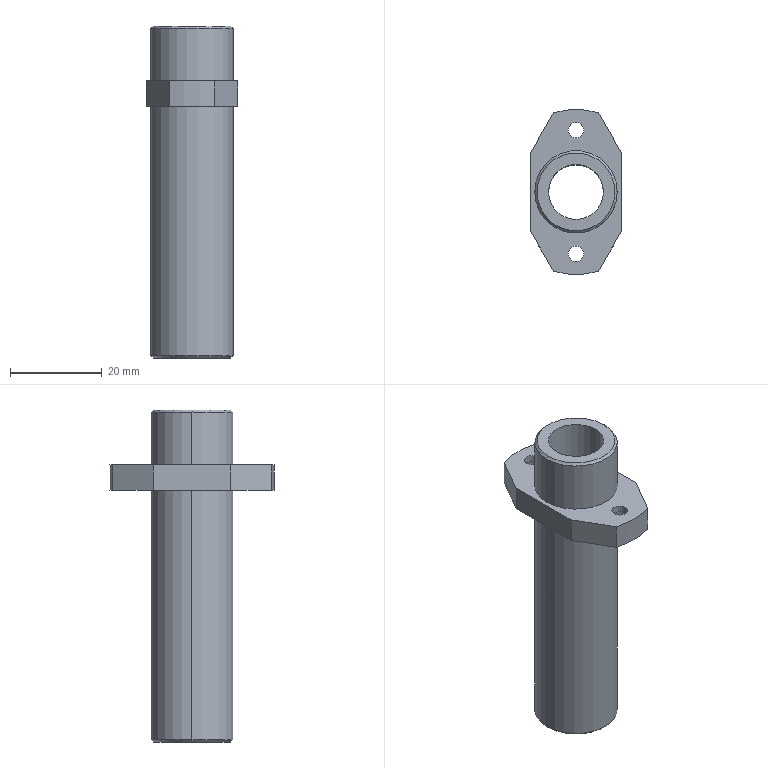Part | STEP file | PN_0016 Default | 1 solid | 38 faces | box 20 x 36 x 72.5 mm | volume 11823 mm3 | cylinder 16 | plane 12 | cone 6 | torus 4 | commonest cylinder face diameters 3.4 x4 6.5 x4 18 x4 12 x2 36 x2
STEP:
#1=CARTESIAN_POINT('',(-7.356,0.,-59.75));
#2=VERTEX_POINT('',#1);
#3=CARTESIAN_POINT('',(7.356,0.,-59.75));
#4=VERTEX_POINT('',#3);
#5=CARTESIAN_POINT('',(0.,0.,-59.75));
#6=DIRECTION('',(0.,0.,-1.));
#7=DIRECTION('',(1.,0.,0.));
#8=AXIS2_PLACEMENT_3D('',#5,#6,#7);
#9=CIRCLE('',#8,7.356);
#10=EDGE_CURVE('',#2,#4,#9,.T.);
#11=ORIENTED_EDGE('',*,*,#10,.F.);
#12=CARTESIAN_POINT('',(-7.789,0.,-60.));
#13=VERTEX_POINT('',#12);
#14=CARTESIAN_POINT('',(-7.789,0.,-59.5));
#15=DIRECTION('',(0.,1.,0.));
#16=DIRECTION('',(-1.,0.,0.));
#17=AXIS2_PLACEMENT_3D('',#14,#15,#16);
#18=CIRCLE('',#17,0.5);
#19=EDGE_CURVE('',#2,#13,#18,.T.);
#20=ORIENTED_EDGE('',*,*,#19,.T.);
#21=CARTESIAN_POINT('',(7.789,0.,-60.));
#22=VERTEX_POINT('',#21);
#23=CARTESIAN_POINT('',(0.,0.,-60.));
#24=DIRECTION('',(0.,0.,1.));
#25=DIRECTION('',(1.,0.,0.));
#26=AXIS2_PLACEMENT_3D('',#23,#24,#25);
#27=CIRCLE('',#26,7.789);
#28=EDGE_CURVE('',#22,#13,#27,.T.);
#29=ORIENTED_EDGE('',*,*,#28,.F.);
#30=CARTESIAN_POINT('',(7.789,0.,-59.5));
#31=DIRECTION('',(0.,-1.,0.));
#32=DIRECTION('',(0.,0.,-1.));
#33=AXIS2_PLACEMENT_3D('',#30,#31,#32);
#34=CIRCLE('',#33,0.5);
#35=EDGE_CURVE('',#4,#22,#34,.T.);
#36=ORIENTED_EDGE('',*,*,#35,.F.);
#37=EDGE_LOOP('',(#11,#20,#29,#36));
#38=FACE_OUTER_BOUND('',#37,.T.);
#39=CARTESIAN_POINT('',(0.,0.,-59.5));
#40=DIRECTION('',(0.,0.,1.));
#41=DIRECTION('',(1.,0.,0.));
#42=AXIS2_PLACEMENT_3D('',#39,#40,#41);
#43=TOROIDAL_SURFACE('',#42,7.789,0.5);
#44=ADVANCED_FACE('',(#38),#43,.T.);
#45=CARTESIAN_POINT('',(6.402,0.,-58.098));
#46=VERTEX_POINT('',#45);
#47=CARTESIAN_POINT('',(-6.402,0.,-58.098));
#48=VERTEX_POINT('',#47);
#49=CARTESIAN_POINT('',(0.,0.,-58.098));
#50=DIRECTION('',(0.,0.,1.));
#51=DIRECTION('',(1.,0.,0.));
#52=AXIS2_PLACEMENT_3D('',#49,#50,#51);
#53=CIRCLE('',#52,6.402);
#54=EDGE_CURVE('',#46,#48,#53,.T.);
#55=ORIENTED_EDGE('',*,*,#54,.F.);
#56=CARTESIAN_POINT('',(6.,0.,-56.598));
#57=VERTEX_POINT('',#56);
#58=CARTESIAN_POINT('',(9.,0.,-56.598));
#59=DIRECTION('',(0.,1.,0.));
#60=DIRECTION('',(-1.,0.,0.));
#61=AXIS2_PLACEMENT_3D('',#58,#59,#60);
#62=CIRCLE('',#61,3.);
#63=EDGE_CURVE('',#46,#57,#62,.T.);
#64=ORIENTED_EDGE('',*,*,#63,.T.);
#65=CARTESIAN_POINT('',(-6.,0.,-56.598));
#66=VERTEX_POINT('',#65);
#67=CARTESIAN_POINT('',(0.,0.,-56.598));
#68=DIRECTION('',(0.,0.,-1.));
#69=DIRECTION('',(-1.,0.,0.));
#70=AXIS2_PLACEMENT_3D('',#67,#68,#69);
#71=CIRCLE('',#70,6.);
#72=EDGE_CURVE('',#66,#57,#71,.T.);
#73=ORIENTED_EDGE('',*,*,#72,.F.);
#74=CARTESIAN_POINT('',(-9.,0.,-56.598));
#75=DIRECTION('',(0.,-1.,0.));
#76=DIRECTION('',(0.,0.,-1.));
#77=AXIS2_PLACEMENT_3D('',#74,#75,#76);
#78=CIRCLE('',#77,3.);
#79=EDGE_CURVE('',#48,#66,#78,.T.);
#80=ORIENTED_EDGE('',*,*,#79,.F.);
#81=EDGE_LOOP('',(#55,#64,#73,#80));
#82=FACE_OUTER_BOUND('',#81,.T.);
#83=CARTESIAN_POINT('',(0.,0.,-56.598));
#84=DIRECTION('',(0.,0.,-1.));
#85=DIRECTION('',(-1.,0.,0.));
#86=AXIS2_PLACEMENT_3D('',#83,#84,#85);
#87=TOROIDAL_SURFACE('',#86,9.,3.);
#88=ADVANCED_FACE('',(#82),#87,.T.);
#89=CARTESIAN_POINT('',(8.5,0.,12.5));
#90=VERTEX_POINT('',#89);
#91=CARTESIAN_POINT('',(-8.5,0.,12.5));
#92=VERTEX_POINT('',#91);
#93=CARTESIAN_POINT('',(0.,0.,12.5));
#94=DIRECTION('',(0.,0.,1.));
#95=DIRECTION('',(-1.,0.,0.));
#96=AXIS2_PLACEMENT_3D('',#93,#94,#95);
#97=CIRCLE('',#96,8.5);
#98=EDGE_CURVE('',#90,#92,#97,.T.);
#99=ORIENTED_EDGE('',*,*,#98,.F.);
#100=CARTESIAN_POINT('',(9.,0.,12.));
#101=VERTEX_POINT('',#100);
#102=CARTESIAN_POINT('',(8.5,0.,12.5));
#103=DIRECTION('',(0.7071,0.,-0.7071));
#104=VECTOR('',#103,1000.);
#105=LINE('',#102,#104);
#106=EDGE_CURVE('',#90,#101,#105,.T.);
#107=ORIENTED_EDGE('',*,*,#106,.T.);
#108=CARTESIAN_POINT('',(-9.,0.,12.));
#109=VERTEX_POINT('',#108);
#110=CARTESIAN_POINT('',(0.,0.,12.));
#111=DIRECTION('',(0.,0.,-1.));
#112=DIRECTION('',(-1.,0.,0.));
#113=AXIS2_PLACEMENT_3D('',#110,#111,#112);
#114=CIRCLE('',#113,9.);
#115=EDGE_CURVE('',#109,#101,#114,.T.);
#116=ORIENTED_EDGE('',*,*,#115,.F.);
#117=CARTESIAN_POINT('',(-8.5,0.,12.5));
#118=DIRECTION('',(-0.7071,0.,-0.7071));
#119=VECTOR('',#118,1000.);
#120=LINE('',#117,#119);
#121=EDGE_CURVE('',#92,#109,#120,.T.);
#122=ORIENTED_EDGE('',*,*,#121,.F.);
#123=EDGE_LOOP('',(#99,#107,#116,#122));
#124=FACE_OUTER_BOUND('',#123,.T.);
#125=CARTESIAN_POINT('',(0.,0.,12.5));
#126=DIRECTION('',(0.,0.,-1.));
#127=DIRECTION('',(-1.,0.,0.));
#128=AXIS2_PLACEMENT_3D('',#125,#126,#127);
#129=CONICAL_SURFACE('',#128,8.5,0.7854);
#130=ADVANCED_FACE('',(#124),#129,.T.);
#131=CARTESIAN_POINT('',(-8.5,0.,-60.));
#132=VERTEX_POINT('',#131);
#133=CARTESIAN_POINT('',(8.5,0.,-60.));
#134=VERTEX_POINT('',#133);
#135=CARTESIAN_POINT('',(0.,0.,-60.));
#136=DIRECTION('',(0.,0.,-1.));
#137=DIRECTION('',(1.,0.,0.));
#138=AXIS2_PLACEMENT_3D('',#135,#136,#137);
#139=CIRCLE('',#138,8.5);
#140=EDGE_CURVE('',#132,#134,#139,.T.);
#141=ORIENTED_EDGE('',*,*,#140,.F.);
#142=CARTESIAN_POINT('',(-9.,0.,-59.5));
#143=VERTEX_POINT('',#142);
#144=CARTESIAN_POINT('',(-9.,0.,-59.5));
#145=DIRECTION('',(-0.7071,0.,0.7071));
#146=VECTOR('',#145,1000.);
#147=LINE('',#144,#146);
#148=EDGE_CURVE('',#132,#143,#147,.T.);
#149=ORIENTED_EDGE('',*,*,#148,.T.);
#150=CARTESIAN_POINT('',(9.,0.,-59.5));
#151=VERTEX_POINT('',#150);
#152=CARTESIAN_POINT('',(0.,0.,-59.5));
#153=DIRECTION('',(0.,0.,1.));
#154=DIRECTION('',(1.,0.,0.));
#155=AXIS2_PLACEMENT_3D('',#152,#153,#154);
#156=CIRCLE('',#155,9.);
#157=EDGE_CURVE('',#151,#143,#156,.T.);
#158=ORIENTED_EDGE('',*,*,#157,.F.);
#159=CARTESIAN_POINT('',(9.,0.,-59.5));
#160=DIRECTION('',(0.7071,0.,0.7071));
#161=VECTOR('',#160,1000.);
#162=LINE('',#159,#161);
#163=EDGE_CURVE('',#134,#151,#162,.T.);
#164=ORIENTED_EDGE('',*,*,#163,.F.);
#165=EDGE_LOOP('',(#141,#149,#158,#164));
#166=FACE_OUTER_BOUND('',#165,.T.);
#167=CARTESIAN_POINT('',(0.,0.,-59.5));
#168=DIRECTION('',(0.,0.,1.));
#169=DIRECTION('',(1.,0.,0.));
#170=AXIS2_PLACEMENT_3D('',#167,#168,#169);
#171=CONICAL_SURFACE('',#170,9.,0.7854);
#172=ADVANCED_FACE('',(#166),#171,.T.);
#173=CARTESIAN_POINT('',(3.25,-13.5,-1.));
#174=VERTEX_POINT('',#173);
#175=CARTESIAN_POINT('',(-3.25,-13.5,-1.));
#176=VERTEX_POINT('',#175);
#177=CARTESIAN_POINT('',(0.,-13.5,-1.));
#178=DIRECTION('',(0.,0.,-1.));
#179=DIRECTION('',(-1.,0.,0.));
#180=AXIS2_PLACEMENT_3D('',#177,#178,#179);
#181=CIRCLE('',#180,3.25);
#182=EDGE_CURVE('',#174,#176,#181,.T.);
#183=ORIENTED_EDGE('',*,*,#182,.F.);
#184=CARTESIAN_POINT('',(3.25,-13.5,-5.));
#185=VERTEX_POINT('',#184);
#186=CARTESIAN_POINT('',(3.25,-13.5,-5.));
#187=DIRECTION('',(0.,0.,-1.));
#188=VECTOR('',#187,1000.);
#189=LINE('',#186,#188);
#190=EDGE_CURVE('',#174,#185,#189,.T.);
#191=ORIENTED_EDGE('',*,*,#190,.T.);
#192=CARTESIAN_POINT('',(-3.25,-13.5,-5.));
#193=VERTEX_POINT('',#192);
#194=CARTESIAN_POINT('',(0.,-13.5,-5.));
#195=DIRECTION('',(0.,0.,-1.));
#196=DIRECTION('',(-1.,0.,0.));
#197=AXIS2_PLACEMENT_3D('',#194,#195,#196);
#198=CIRCLE('',#197,3.25);
#199=EDGE_CURVE('',#185,#193,#198,.T.);
#200=ORIENTED_EDGE('',*,*,#199,.T.);
#201=CARTESIAN_POINT('',(-3.25,-13.5,-5.));
#202=DIRECTION('',(0.,0.,-1.));
#203=VECTOR('',#202,1000.);
#204=LINE('',#201,#203);
#205=EDGE_CURVE('',#176,#193,#204,.T.);
#206=ORIENTED_EDGE('',*,*,#205,.F.);
#207=EDGE_LOOP('',(#183,#191,#200,#206));
#208=FACE_OUTER_BOUND('',#207,.T.);
#209=CARTESIAN_POINT('',(0.,-13.5,-5.));
#210=DIRECTION('',(0.,0.,-1.));
#211=DIRECTION('',(-1.,0.,0.));
#212=AXIS2_PLACEMENT_3D('',#209,#210,#211);
#213=CYLINDRICAL_SURFACE('',#212,3.25);
#214=ADVANCED_FACE('',(#208),#213,.F.);
#215=CARTESIAN_POINT('',(1.7,-13.5,0.5));
#216=VERTEX_POINT('',#215);
#217=CARTESIAN_POINT('',(-1.7,-13.5,0.5));
#218=VERTEX_POINT('',#217);
#219=CARTESIAN_POINT('',(0.,-13.5,0.5));
#220=DIRECTION('',(0.,0.,-1.));
#221=DIRECTION('',(-1.,0.,0.));
#222=AXIS2_PLACEMENT_3D('',#219,#220,#221);
#223=CIRCLE('',#222,1.7);
#224=EDGE_CURVE('',#216,#218,#223,.T.);
#225=ORIENTED_EDGE('',*,*,#224,.F.);
#226=CARTESIAN_POINT('',(1.7,-13.5,-1.));
#227=VERTEX_POINT('',#226);
#228=CARTESIAN_POINT('',(1.7,-13.5,-5.));
#229=DIRECTION('',(0.,0.,-1.));
#230=VECTOR('',#229,1000.);
#231=LINE('',#228,#230);
#232=EDGE_CURVE('',#216,#227,#231,.T.);
#233=ORIENTED_EDGE('',*,*,#232,.T.);
#234=CARTESIAN_POINT('',(-1.7,-13.5,-1.));
#235=VERTEX_POINT('',#234);
#236=CARTESIAN_POINT('',(0.,-13.5,-1.));
#237=DIRECTION('',(0.,0.,-1.));
#238=DIRECTION('',(-1.,0.,0.));
#239=AXIS2_PLACEMENT_3D('',#236,#237,#238);
#240=CIRCLE('',#239,1.7);
#241=EDGE_CURVE('',#227,#235,#240,.T.);
#242=ORIENTED_EDGE('',*,*,#241,.T.);
#243=CARTESIAN_POINT('',(-1.7,-13.5,-5.));
#244=DIRECTION('',(0.,0.,-1.));
#245=VECTOR('',#244,1000.);
#246=LINE('',#243,#245);
#247=EDGE_CURVE('',#218,#235,#246,.T.);
#248=ORIENTED_EDGE('',*,*,#247,.F.);
#249=EDGE_LOOP('',(#225,#233,#242,#248));
#250=FACE_OUTER_BOUND('',#249,.T.);
#251=CARTESIAN_POINT('',(0.,-13.5,-5.));
#252=DIRECTION('',(0.,0.,-1.));
#253=DIRECTION('',(-1.,0.,0.));
#254=AXIS2_PLACEMENT_3D('',#251,#252,#253);
#255=CYLINDRICAL_SURFACE('',#254,1.7);
#256=ADVANCED_FACE('',(#250),#255,.F.);
#257=CARTESIAN_POINT('',(3.25,13.5,-1.));
#258=VERTEX_POINT('',#257);
#259=CARTESIAN_POINT('',(-3.25,13.5,-1.));
#260=VERTEX_POINT('',#259);
#261=CARTESIAN_POINT('',(0.,13.5,-1.));
#262=DIRECTION('',(0.,0.,-1.));
#263=DIRECTION('',(-1.,0.,0.));
#264=AXIS2_PLACEMENT_3D('',#261,#262,#263);
#265=CIRCLE('',#264,3.25);
#266=EDGE_CURVE('',#258,#260,#265,.T.);
#267=ORIENTED_EDGE('',*,*,#266,.F.);
#268=CARTESIAN_POINT('',(3.25,13.5,-5.));
#269=VERTEX_POINT('',#268);
#270=CARTESIAN_POINT('',(3.25,13.5,-5.));
#271=DIRECTION('',(0.,0.,-1.));
#272=VECTOR('',#271,1000.);
#273=LINE('',#270,#272);
#274=EDGE_CURVE('',#258,#269,#273,.T.);
#275=ORIENTED_EDGE('',*,*,#274,.T.);
#276=CARTESIAN_POINT('',(-3.25,13.5,-5.));
#277=VERTEX_POINT('',#276);
#278=CARTESIAN_POINT('',(0.,13.5,-5.));
#279=DIRECTION('',(0.,0.,-1.));
#280=DIRECTION('',(-1.,0.,0.));
#281=AXIS2_PLACEMENT_3D('',#278,#279,#280);
#282=CIRCLE('',#281,3.25);
#283=EDGE_CURVE('',#269,#277,#282,.T.);
#284=ORIENTED_EDGE('',*,*,#283,.T.);
#285=CARTESIAN_POINT('',(-3.25,13.5,-5.));
#286=DIRECTION('',(0.,0.,-1.));
#287=VECTOR('',#286,1000.);
#288=LINE('',#285,#287);
#289=EDGE_CURVE('',#260,#277,#288,.T.);
#290=ORIENTED_EDGE('',*,*,#289,.F.);
#291=EDGE_LOOP('',(#267,#275,#284,#290));
#292=FACE_OUTER_BOUND('',#291,.T.);
#293=CARTESIAN_POINT('',(0.,13.5,-5.));
#294=DIRECTION('',(0.,0.,-1.));
#295=DIRECTION('',(-1.,0.,0.));
#296=AXIS2_PLACEMENT_3D('',#293,#294,#295);
#297=CYLINDRICAL_SURFACE('',#296,3.25);
#298=ADVANCED_FACE('',(#292),#297,.F.);
#299=CARTESIAN_POINT('',(1.7,13.5,0.5));
#300=VERTEX_POINT('',#299);
#301=CARTESIAN_POINT('',(-1.7,13.5,0.5));
#302=VERTEX_POINT('',#301);
#303=CARTESIAN_POINT('',(0.,13.5,0.5));
#304=DIRECTION('',(0.,0.,-1.));
#305=DIRECTION('',(-1.,0.,0.));
#306=AXIS2_PLACEMENT_3D('',#303,#304,#305);
#307=CIRCLE('',#306,1.7);
#308=EDGE_CURVE('',#300,#302,#307,.T.);
#309=ORIENTED_EDGE('',*,*,#308,.F.);
#310=CARTESIAN_POINT('',(1.7,13.5,-1.));
#311=VERTEX_POINT('',#310);
#312=CARTESIAN_POINT('',(1.7,13.5,-5.));
#313=DIRECTION('',(0.,0.,-1.));
#314=VECTOR('',#313,1000.);
#315=LINE('',#312,#314);
#316=EDGE_CURVE('',#300,#311,#315,.T.);
#317=ORIENTED_EDGE('',*,*,#316,.T.);
#318=CARTESIAN_POINT('',(-1.7,13.5,-1.));
#319=VERTEX_POINT('',#318);
#320=CARTESIAN_POINT('',(0.,13.5,-1.));
#321=DIRECTION('',(0.,0.,-1.));
#322=DIRECTION('',(-1.,0.,0.));
#323=AXIS2_PLACEMENT_3D('',#320,#321,#322);
#324=CIRCLE('',#323,1.7);
#325=EDGE_CURVE('',#311,#319,#324,.T.);
#326=ORIENTED_EDGE('',*,*,#325,.T.);
#327=CARTESIAN_POINT('',(-1.7,13.5,-5.));
#328=DIRECTION('',(0.,0.,-1.));
#329=VECTOR('',#328,1000.);
#330=LINE('',#327,#329);
#331=EDGE_CURVE('',#302,#319,#330,.T.);
#332=ORIENTED_EDGE('',*,*,#331,.F.);
#333=EDGE_LOOP('',(#309,#317,#326,#332));
#334=FACE_OUTER_BOUND('',#333,.T.);
#335=CARTESIAN_POINT('',(0.,13.5,-5.));
#336=DIRECTION('',(0.,0.,-1.));
#337=DIRECTION('',(-1.,0.,0.));
#338=AXIS2_PLACEMENT_3D('',#335,#336,#337);
#339=CYLINDRICAL_SURFACE('',#338,1.7);
#340=ADVANCED_FACE('',(#334),#339,.F.);
#341=ORIENTED_EDGE('',*,*,#157,.T.);
#342=CARTESIAN_POINT('',(-9.,0.,-5.));
#343=VERTEX_POINT('',#342);
#344=CARTESIAN_POINT('',(-9.,0.,0.));
#345=DIRECTION('',(0.,0.,1.));
#346=VECTOR('',#345,1000.);
#347=LINE('',#344,#346);
#348=EDGE_CURVE('',#143,#343,#347,.T.);
#349=ORIENTED_EDGE('',*,*,#348,.T.);
#350=CARTESIAN_POINT('',(9.,0.,-5.));
#351=VERTEX_POINT('',#350);
#352=CARTESIAN_POINT('',(0.,0.,-5.));
#353=DIRECTION('',(0.,0.,1.));
#354=DIRECTION('',(1.,0.,0.));
#355=AXIS2_PLACEMENT_3D('',#352,#353,#354);
#356=CIRCLE('',#355,9.);
#357=EDGE_CURVE('',#351,#343,#356,.T.);
#358=ORIENTED_EDGE('',*,*,#357,.F.);
#359=CARTESIAN_POINT('',(9.,0.,0.));
#360=DIRECTION('',(0.,0.,1.));
#361=VECTOR('',#360,1000.);
#362=LINE('',#359,#361);
#363=EDGE_CURVE('',#151,#351,#362,.T.);
#364=ORIENTED_EDGE('',*,*,#363,.F.);
#365=EDGE_LOOP('',(#341,#349,#358,#364));
#366=FACE_OUTER_BOUND('',#365,.T.);
#367=CARTESIAN_POINT('',(0.,0.,0.));
#368=DIRECTION('',(0.,0.,1.));
#369=DIRECTION('',(1.,0.,0.));
#370=AXIS2_PLACEMENT_3D('',#367,#368,#369);
#371=CYLINDRICAL_SURFACE('',#370,9.);
#372=ADVANCED_FACE('',(#366),#371,.T.);
#373=CARTESIAN_POINT('',(0.,0.,-58.098));
#374=DIRECTION('',(0.,0.,1.));
#375=DIRECTION('',(1.,0.,0.));
#376=AXIS2_PLACEMENT_3D('',#373,#374,#375);
#377=CIRCLE('',#376,6.402);
#378=EDGE_CURVE('',#48,#46,#377,.T.);
#379=ORIENTED_EDGE('',*,*,#378,.T.);
#380=CARTESIAN_POINT('',(6.,0.,-57.402));
#381=DIRECTION('',(0.5,0.,-0.866));
#382=VECTOR('',#381,1000.);
#383=LINE('',#380,#382);
#384=EDGE_CURVE('',#46,#4,#383,.T.);
#385=ORIENTED_EDGE('',*,*,#384,.T.);
#386=CARTESIAN_POINT('',(0.,0.,-59.75));
#387=DIRECTION('',(0.,0.,-1.));
#388=DIRECTION('',(1.,0.,0.));
#389=AXIS2_PLACEMENT_3D('',#386,#387,#388);
#390=CIRCLE('',#389,7.356);
#391=EDGE_CURVE('',#4,#2,#390,.T.);
#392=ORIENTED_EDGE('',*,*,#391,.T.);
#393=CARTESIAN_POINT('',(-6.,0.,-57.402));
#394=DIRECTION('',(-0.5,0.,-0.866));
#395=VECTOR('',#394,1000.);
#396=LINE('',#393,#395);
#397=EDGE_CURVE('',#48,#2,#396,.T.);
#398=ORIENTED_EDGE('',*,*,#397,.F.);
#399=EDGE_LOOP('',(#379,#385,#392,#398));
#400=FACE_OUTER_BOUND('',#399,.T.);
#401=CARTESIAN_POINT('',(0.,0.,-57.402));
#402=DIRECTION('',(0.,0.,-1.));
#403=DIRECTION('',(-1.,0.,0.));
#404=AXIS2_PLACEMENT_3D('',#401,#402,#403);
#405=CONICAL_SURFACE('',#404,6.,0.5236);
#406=ADVANCED_FACE('',(#400),#405,.F.);
#407=CARTESIAN_POINT('',(0.,0.,-56.598));
#408=DIRECTION('',(0.,0.,-1.));
#409=DIRECTION('',(-1.,0.,0.));
#410=AXIS2_PLACEMENT_3D('',#407,#408,#409);
#411=CIRCLE('',#410,6.);
#412=EDGE_CURVE('',#57,#66,#411,.T.);
#413=ORIENTED_EDGE('',*,*,#412,.T.);
#414=CARTESIAN_POINT('',(-6.,0.,12.5));
#415=VERTEX_POINT('',#414);
#416=CARTESIAN_POINT('',(-6.,0.,0.));
#417=DIRECTION('',(0.,0.,1.));
#418=VECTOR('',#417,1000.);
#419=LINE('',#416,#418);
#420=EDGE_CURVE('',#66,#415,#419,.T.);
#421=ORIENTED_EDGE('',*,*,#420,.T.);
#422=CARTESIAN_POINT('',(6.,0.,12.5));
#423=VERTEX_POINT('',#422);
#424=CARTESIAN_POINT('',(0.,0.,12.5));
#425=DIRECTION('',(0.,0.,1.));
#426=DIRECTION('',(1.,0.,0.));
#427=AXIS2_PLACEMENT_3D('',#424,#425,#426);
#428=CIRCLE('',#427,6.);
#429=EDGE_CURVE('',#415,#423,#428,.T.);
#430=ORIENTED_EDGE('',*,*,#429,.T.);
#431=CARTESIAN_POINT('',(6.,0.,0.));
#432=DIRECTION('',(0.,0.,1.));
#433=VECTOR('',#432,1000.);
#434=LINE('',#431,#433);
#435=EDGE_CURVE('',#57,#423,#434,.T.);
#436=ORIENTED_EDGE('',*,*,#435,.F.);
#437=EDGE_LOOP('',(#413,#421,#430,#436));
#438=FACE_OUTER_BOUND('',#437,.T.);
#439=CARTESIAN_POINT('',(0.,0.,0.));
#440=DIRECTION('',(0.,0.,1.));
#441=DIRECTION('',(1.,0.,0.));
#442=AXIS2_PLACEMENT_3D('',#439,#440,#441);
#443=CYLINDRICAL_SURFACE('',#442,6.);
#444=ADVANCED_FACE('',(#438),#443,.F.);
#445=CARTESIAN_POINT('',(9.,0.,0.5));
#446=VERTEX_POINT('',#445);
#447=CARTESIAN_POINT('',(-9.,0.,0.5));
#448=VERTEX_POINT('',#447);
#449=CARTESIAN_POINT('',(0.,0.,0.5));
#450=DIRECTION('',(0.,0.,1.));
#451=DIRECTION('',(1.,0.,0.));
#452=AXIS2_PLACEMENT_3D('',#449,#450,#451);
#453=CIRCLE('',#452,9.);
#454=EDGE_CURVE('',#446,#448,#453,.T.);
#455=ORIENTED_EDGE('',*,*,#454,.T.);
#456=CARTESIAN_POINT('',(-9.,0.,0.));
#457=DIRECTION('',(0.,0.,1.));
#458=VECTOR('',#457,1000.);
#459=LINE('',#456,#458);
#460=EDGE_CURVE('',#448,#109,#459,.T.);
#461=ORIENTED_EDGE('',*,*,#460,.T.);
#462=ORIENTED_EDGE('',*,*,#115,.T.);
#463=CARTESIAN_POINT('',(9.,0.,0.));
#464=DIRECTION('',(0.,0.,1.));
#465=VECTOR('',#464,1000.);
#466=LINE('',#463,#465);
#467=EDGE_CURVE('',#446,#101,#466,.T.);
#468=ORIENTED_EDGE('',*,*,#467,.F.);
#469=EDGE_LOOP('',(#455,#461,#462,#468));
#470=FACE_OUTER_BOUND('',#469,.T.);
#471=CARTESIAN_POINT('',(0.,0.,0.));
#472=DIRECTION('',(0.,0.,1.));
#473=DIRECTION('',(1.,0.,0.));
#474=AXIS2_PLACEMENT_3D('',#471,#472,#473);
#475=CYLINDRICAL_SURFACE('',#474,9.);
#476=ADVANCED_FACE('',(#470),#475,.T.);
#477=CARTESIAN_POINT('',(4.886,17.324,-5.));
#478=VERTEX_POINT('',#477);
#479=CARTESIAN_POINT('',(-4.886,17.324,-5.));
#480=VERTEX_POINT('',#479);
#481=CARTESIAN_POINT('',(0.,0.,-5.));
#482=DIRECTION('',(0.,0.,1.));
#483=DIRECTION('',(1.,0.,0.));
#484=AXIS2_PLACEMENT_3D('',#481,#482,#483);
#485=CIRCLE('',#484,18.);
#486=EDGE_CURVE('',#478,#480,#485,.T.);
#487=ORIENTED_EDGE('',*,*,#486,.T.);
#488=CARTESIAN_POINT('',(-4.886,17.324,0.5));
#489=VERTEX_POINT('',#488);
#490=CARTESIAN_POINT('',(-4.886,17.324,0.));
#491=DIRECTION('',(0.,0.,1.));
#492=VECTOR('',#491,1000.);
#493=LINE('',#490,#492);
#494=EDGE_CURVE('',#480,#489,#493,.T.);
#495=ORIENTED_EDGE('',*,*,#494,.T.);
#496=CARTESIAN_POINT('',(4.886,17.324,0.5));
#497=VERTEX_POINT('',#496);
#498=CARTESIAN_POINT('',(0.,0.,0.5));
#499=DIRECTION('',(0.,0.,1.));
#500=DIRECTION('',(1.,0.,0.));
#501=AXIS2_PLACEMENT_3D('',#498,#499,#500);
#502=CIRCLE('',#501,18.);
#503=EDGE_CURVE('',#497,#489,#502,.T.);
#504=ORIENTED_EDGE('',*,*,#503,.F.);
#505=CARTESIAN_POINT('',(4.886,17.324,0.));
#506=DIRECTION('',(0.,0.,-1.));
#507=VECTOR('',#506,1000.);
#508=LINE('',#505,#507);
#509=EDGE_CURVE('',#497,#478,#508,.T.);
#510=ORIENTED_EDGE('',*,*,#509,.T.);
#511=EDGE_LOOP('',(#487,#495,#504,#510));
#512=FACE_OUTER_BOUND('',#511,.T.);
#513=CARTESIAN_POINT('',(0.,0.,0.));
#514=DIRECTION('',(0.,0.,1.));
#515=DIRECTION('',(1.,0.,0.));
#516=AXIS2_PLACEMENT_3D('',#513,#514,#515);
#517=CYLINDRICAL_SURFACE('',#516,18.);
#518=ADVANCED_FACE('',(#512),#517,.T.);
#519=ORIENTED_EDGE('',*,*,#460,.F.);
#520=CARTESIAN_POINT('',(0.,0.,0.5));
#521=DIRECTION('',(0.,0.,1.));
#522=DIRECTION('',(1.,0.,0.));
#523=AXIS2_PLACEMENT_3D('',#520,#521,#522);
#524=CIRCLE('',#523,9.);
#525=EDGE_CURVE('',#448,#446,#524,.T.);
#526=ORIENTED_EDGE('',*,*,#525,.T.);
#527=ORIENTED_EDGE('',*,*,#467,.T.);
#528=CARTESIAN_POINT('',(0.,0.,12.));
#529=DIRECTION('',(0.,0.,-1.));
#530=DIRECTION('',(-1.,0.,0.));
#531=AXIS2_PLACEMENT_3D('',#528,#529,#530);
#532=CIRCLE('',#531,9.);
#533=EDGE_CURVE('',#101,#109,#532,.T.);
#534=ORIENTED_EDGE('',*,*,#533,.T.);
#535=EDGE_LOOP('',(#519,#526,#527,#534));
#536=FACE_OUTER_BOUND('',#535,.T.);
#537=CARTESIAN_POINT('',(0.,0.,0.));
#538=DIRECTION('',(0.,0.,1.));
#539=DIRECTION('',(1.,0.,0.));
#540=AXIS2_PLACEMENT_3D('',#537,#538,#539);
#541=CYLINDRICAL_SURFACE('',#540,9.);
#542=ADVANCED_FACE('',(#536),#541,.T.);
#543=CARTESIAN_POINT('',(0.,0.,12.5));
#544=DIRECTION('',(0.,0.,1.));
#545=DIRECTION('',(-1.,0.,0.));
#546=AXIS2_PLACEMENT_3D('',#543,#544,#545);
#547=CIRCLE('',#546,8.5);
#548=EDGE_CURVE('',#92,#90,#547,.T.);
#549=ORIENTED_EDGE('',*,*,#548,.T.);
#550=ORIENTED_EDGE('',*,*,#98,.T.);
#551=EDGE_LOOP('',(#549,#550));
#552=FACE_OUTER_BOUND('',#551,.T.);
#553=CARTESIAN_POINT('',(0.,0.,12.5));
#554=DIRECTION('',(0.,0.,1.));
#555=DIRECTION('',(1.,0.,0.));
#556=AXIS2_PLACEMENT_3D('',#553,#554,#555);
#557=CIRCLE('',#556,6.);
#558=EDGE_CURVE('',#423,#415,#557,.T.);
#559=ORIENTED_EDGE('',*,*,#558,.F.);
#560=ORIENTED_EDGE('',*,*,#429,.F.);
#561=EDGE_LOOP('',(#559,#560));
#562=FACE_BOUND('',#561,.T.);
#563=CARTESIAN_POINT('',(-6.,0.,12.5));
#564=DIRECTION('',(0.,0.,-1.));
#565=DIRECTION('',(-1.,0.,0.));
#566=AXIS2_PLACEMENT_3D('',#563,#564,#565);
#567=PLANE('',#566);
#568=ADVANCED_FACE('',(#552,#562),#567,.F.);
#569=ORIENTED_EDGE('',*,*,#420,.F.);
#570=ORIENTED_EDGE('',*,*,#72,.T.);
#571=ORIENTED_EDGE('',*,*,#435,.T.);
#572=ORIENTED_EDGE('',*,*,#558,.T.);
#573=EDGE_LOOP('',(#569,#570,#571,#572));
#574=FACE_OUTER_BOUND('',#573,.T.);
#575=CARTESIAN_POINT('',(0.,0.,0.));
#576=DIRECTION('',(0.,0.,1.));
#577=DIRECTION('',(1.,0.,0.));
#578=AXIS2_PLACEMENT_3D('',#575,#576,#577);
#579=CYLINDRICAL_SURFACE('',#578,6.);
#580=ADVANCED_FACE('',(#574),#579,.F.);
#581=ORIENTED_EDGE('',*,*,#384,.F.);
#582=ORIENTED_EDGE('',*,*,#54,.T.);
#583=ORIENTED_EDGE('',*,*,#397,.T.);
#584=ORIENTED_EDGE('',*,*,#10,.T.);
#585=EDGE_LOOP('',(#581,#582,#583,#584));
#586=FACE_OUTER_BOUND('',#585,.T.);
#587=CARTESIAN_POINT('',(0.,0.,-57.402));
#588=DIRECTION('',(0.,0.,-1.));
#589=DIRECTION('',(-1.,0.,0.));
#590=AXIS2_PLACEMENT_3D('',#587,#588,#589);
#591=CONICAL_SURFACE('',#590,6.,0.5236);
#592=ADVANCED_FACE('',(#586),#591,.F.);
#593=ORIENTED_EDGE('',*,*,#28,.T.);
#594=CARTESIAN_POINT('',(0.,0.,-60.));
#595=DIRECTION('',(0.,0.,1.));
#596=DIRECTION('',(1.,0.,0.));
#597=AXIS2_PLACEMENT_3D('',#594,#595,#596);
#598=CIRCLE('',#597,7.789);
#599=EDGE_CURVE('',#13,#22,#598,.T.);
#600=ORIENTED_EDGE('',*,*,#599,.T.);
#601=EDGE_LOOP('',(#593,#600));
#602=FACE_BOUND('',#601,.T.);
#603=CARTESIAN_POINT('',(0.,0.,-60.));
#604=DIRECTION('',(0.,0.,-1.));
#605=DIRECTION('',(1.,0.,0.));
#606=AXIS2_PLACEMENT_3D('',#603,#604,#605);
#607=CIRCLE('',#606,8.5);
#608=EDGE_CURVE('',#134,#132,#607,.T.);
#609=ORIENTED_EDGE('',*,*,#608,.T.);
#610=ORIENTED_EDGE('',*,*,#140,.T.);
#611=EDGE_LOOP('',(#609,#610));
#612=FACE_OUTER_BOUND('',#611,.T.);
#613=CARTESIAN_POINT('',(-9.,0.,-60.));
#614=DIRECTION('',(0.,0.,1.));
#615=DIRECTION('',(1.,0.,0.));
#616=AXIS2_PLACEMENT_3D('',#613,#614,#615);
#617=PLANE('',#616);
#618=ADVANCED_FACE('',(#602,#612),#617,.F.);
#619=ORIENTED_EDGE('',*,*,#348,.F.);
#620=CARTESIAN_POINT('',(0.,0.,-59.5));
#621=DIRECTION('',(0.,0.,1.));
#622=DIRECTION('',(1.,0.,0.));
#623=AXIS2_PLACEMENT_3D('',#620,#621,#622);
#624=CIRCLE('',#623,9.);
#625=EDGE_CURVE('',#143,#151,#624,.T.);
#626=ORIENTED_EDGE('',*,*,#625,.T.);
#627=ORIENTED_EDGE('',*,*,#363,.T.);
#628=CARTESIAN_POINT('',(0.,0.,-5.));
#629=DIRECTION('',(0.,0.,1.));
#630=DIRECTION('',(1.,0.,0.));
#631=AXIS2_PLACEMENT_3D('',#628,#629,#630);
#632=CIRCLE('',#631,9.);
#633=EDGE_CURVE('',#343,#351,#632,.T.);
#634=ORIENTED_EDGE('',*,*,#633,.F.);
#635=EDGE_LOOP('',(#619,#626,#627,#634));
#636=FACE_OUTER_BOUND('',#635,.T.);
#637=CARTESIAN_POINT('',(0.,0.,0.));
#638=DIRECTION('',(0.,0.,1.));
#639=DIRECTION('',(1.,0.,0.));
#640=AXIS2_PLACEMENT_3D('',#637,#638,#639);
#641=CYLINDRICAL_SURFACE('',#640,9.);
#642=ADVANCED_FACE('',(#636),#641,.T.);
#643=CARTESIAN_POINT('',(0.,-13.5,-5.));
#644=DIRECTION('',(0.,0.,-1.));
#645=DIRECTION('',(-1.,0.,0.));
#646=AXIS2_PLACEMENT_3D('',#643,#644,#645);
#647=CIRCLE('',#646,3.25);
#648=EDGE_CURVE('',#193,#185,#647,.T.);
#649=ORIENTED_EDGE('',*,*,#648,.F.);
#650=ORIENTED_EDGE('',*,*,#199,.F.);
#651=EDGE_LOOP('',(#649,#650));
#652=FACE_BOUND('',#651,.T.);
#653=CARTESIAN_POINT('',(0.,13.5,-5.));
#654=DIRECTION('',(0.,0.,-1.));
#655=DIRECTION('',(-1.,0.,0.));
#656=AXIS2_PLACEMENT_3D('',#653,#654,#655);
#657=CIRCLE('',#656,3.25);
#658=EDGE_CURVE('',#277,#269,#657,.T.);
#659=ORIENTED_EDGE('',*,*,#658,.F.);
#660=ORIENTED_EDGE('',*,*,#283,.F.);
#661=EDGE_LOOP('',(#659,#660));
#662=FACE_BOUND('',#661,.T.);
#663=CARTESIAN_POINT('',(10.,-8.467,-5.));
#664=VERTEX_POINT('',#663);
#665=CARTESIAN_POINT('',(10.,8.467,-5.));
#666=VERTEX_POINT('',#665);
#667=CARTESIAN_POINT('',(10.,20.374,-5.));
#668=DIRECTION('',(0.,1.,0.));
#669=VECTOR('',#668,1000.);
#670=LINE('',#667,#669);
#671=EDGE_CURVE('',#664,#666,#670,.T.);
#672=ORIENTED_EDGE('',*,*,#671,.F.);
#673=CARTESIAN_POINT('',(4.886,-17.324,-5.));
#674=VERTEX_POINT('',#673);
#675=CARTESIAN_POINT('',(4.886,-17.324,-5.));
#676=DIRECTION('',(-0.5,-0.866,0.));
#677=VECTOR('',#676,1000.);
#678=LINE('',#675,#677);
#679=EDGE_CURVE('',#664,#674,#678,.T.);
#680=ORIENTED_EDGE('',*,*,#679,.T.);
#681=CARTESIAN_POINT('',(-4.886,-17.324,-5.));
#682=VERTEX_POINT('',#681);
#683=CARTESIAN_POINT('',(0.,0.,-5.));
#684=DIRECTION('',(0.,0.,1.));
#685=DIRECTION('',(1.,0.,0.));
#686=AXIS2_PLACEMENT_3D('',#683,#684,#685);
#687=CIRCLE('',#686,18.);
#688=EDGE_CURVE('',#682,#674,#687,.T.);
#689=ORIENTED_EDGE('',*,*,#688,.F.);
#690=CARTESIAN_POINT('',(-10.,-8.467,-5.));
#691=VERTEX_POINT('',#690);
#692=CARTESIAN_POINT('',(-4.886,-17.324,-5.));
#693=DIRECTION('',(-0.5,0.866,0.));
#694=VECTOR('',#693,1000.);
#695=LINE('',#692,#694);
#696=EDGE_CURVE('',#682,#691,#695,.T.);
#697=ORIENTED_EDGE('',*,*,#696,.T.);
#698=CARTESIAN_POINT('',(-10.,8.467,-5.));
#699=VERTEX_POINT('',#698);
#700=CARTESIAN_POINT('',(-10.,20.374,-5.));
#701=DIRECTION('',(0.,-1.,0.));
#702=VECTOR('',#701,1000.);
#703=LINE('',#700,#702);
#704=EDGE_CURVE('',#699,#691,#703,.T.);
#705=ORIENTED_EDGE('',*,*,#704,.F.);
#706=CARTESIAN_POINT('',(-4.886,17.324,-5.));
#707=DIRECTION('',(0.5,0.866,0.));
#708=VECTOR('',#707,1000.);
#709=LINE('',#706,#708);
#710=EDGE_CURVE('',#699,#480,#709,.T.);
#711=ORIENTED_EDGE('',*,*,#710,.T.);
#712=ORIENTED_EDGE('',*,*,#486,.F.);
#713=CARTESIAN_POINT('',(4.886,17.324,-5.));
#714=DIRECTION('',(0.5,-0.866,0.));
#715=VECTOR('',#714,1000.);
#716=LINE('',#713,#715);
#717=EDGE_CURVE('',#478,#666,#716,.T.);
#718=ORIENTED_EDGE('',*,*,#717,.T.);
#719=EDGE_LOOP('',(#672,#680,#689,#697,#705,#711,#712,#718));
#720=FACE_OUTER_BOUND('',#719,.T.);
#721=ORIENTED_EDGE('',*,*,#357,.T.);
#722=ORIENTED_EDGE('',*,*,#633,.T.);
#723=EDGE_LOOP('',(#721,#722));
#724=FACE_BOUND('',#723,.T.);
#725=CARTESIAN_POINT('',(-18.,0.,-5.));
#726=DIRECTION('',(0.,0.,1.));
#727=DIRECTION('',(1.,0.,0.));
#728=AXIS2_PLACEMENT_3D('',#725,#726,#727);
#729=PLANE('',#728);
#730=ADVANCED_FACE('',(#652,#662,#720,#724),#729,.F.);
#731=ORIENTED_EDGE('',*,*,#688,.T.);
#732=CARTESIAN_POINT('',(4.886,-17.324,0.5));
#733=VERTEX_POINT('',#732);
#734=CARTESIAN_POINT('',(4.886,-17.324,0.));
#735=DIRECTION('',(0.,0.,1.));
#736=VECTOR('',#735,1000.);
#737=LINE('',#734,#736);
#738=EDGE_CURVE('',#674,#733,#737,.T.);
#739=ORIENTED_EDGE('',*,*,#738,.T.);
#740=CARTESIAN_POINT('',(-4.886,-17.324,0.5));
#741=VERTEX_POINT('',#740);
#742=CARTESIAN_POINT('',(0.,0.,0.5));
#743=DIRECTION('',(0.,0.,1.));
#744=DIRECTION('',(1.,0.,0.));
#745=AXIS2_PLACEMENT_3D('',#742,#743,#744);
#746=CIRCLE('',#745,18.);
#747=EDGE_CURVE('',#741,#733,#746,.T.);
#748=ORIENTED_EDGE('',*,*,#747,.F.);
#749=CARTESIAN_POINT('',(-4.886,-17.324,0.));
#750=DIRECTION('',(0.,0.,-1.));
#751=VECTOR('',#750,1000.);
#752=LINE('',#749,#751);
#753=EDGE_CURVE('',#741,#682,#752,.T.);
#754=ORIENTED_EDGE('',*,*,#753,.T.);
#755=EDGE_LOOP('',(#731,#739,#748,#754));
#756=FACE_OUTER_BOUND('',#755,.T.);
#757=CARTESIAN_POINT('',(0.,0.,0.));
#758=DIRECTION('',(0.,0.,1.));
#759=DIRECTION('',(1.,0.,0.));
#760=AXIS2_PLACEMENT_3D('',#757,#758,#759);
#761=CYLINDRICAL_SURFACE('',#760,18.);
#762=ADVANCED_FACE('',(#756),#761,.T.);
#763=CARTESIAN_POINT('',(0.,-13.5,0.5));
#764=DIRECTION('',(0.,0.,-1.));
#765=DIRECTION('',(-1.,0.,0.));
#766=AXIS2_PLACEMENT_3D('',#763,#764,#765);
#767=CIRCLE('',#766,1.7);
#768=EDGE_CURVE('',#218,#216,#767,.T.);
#769=ORIENTED_EDGE('',*,*,#768,.T.);
#770=ORIENTED_EDGE('',*,*,#224,.T.);
#771=EDGE_LOOP('',(#769,#770));
#772=FACE_BOUND('',#771,.T.);
#773=CARTESIAN_POINT('',(0.,13.5,0.5));
#774=DIRECTION('',(0.,0.,-1.));
#775=DIRECTION('',(-1.,0.,0.));
#776=AXIS2_PLACEMENT_3D('',#773,#774,#775);
#777=CIRCLE('',#776,1.7);
#778=EDGE_CURVE('',#302,#300,#777,.T.);
#779=ORIENTED_EDGE('',*,*,#778,.T.);
#780=ORIENTED_EDGE('',*,*,#308,.T.);
#781=EDGE_LOOP('',(#779,#780));
#782=FACE_BOUND('',#781,.T.);
#783=ORIENTED_EDGE('',*,*,#454,.F.);
#784=ORIENTED_EDGE('',*,*,#525,.F.);
#785=EDGE_LOOP('',(#783,#784));
#786=FACE_BOUND('',#785,.T.);
#787=ORIENTED_EDGE('',*,*,#747,.T.);
#788=CARTESIAN_POINT('',(10.,-8.467,0.5));
#789=VERTEX_POINT('',#788);
#790=CARTESIAN_POINT('',(4.886,-17.324,0.5));
#791=DIRECTION('',(0.5,0.866,0.));
#792=VECTOR('',#791,1000.);
#793=LINE('',#790,#792);
#794=EDGE_CURVE('',#733,#789,#793,.T.);
#795=ORIENTED_EDGE('',*,*,#794,.T.);
#796=CARTESIAN_POINT('',(10.,8.467,0.5));
#797=VERTEX_POINT('',#796);
#798=CARTESIAN_POINT('',(10.,0.,0.5));
#799=DIRECTION('',(0.,1.,0.));
#800=VECTOR('',#799,1000.);
#801=LINE('',#798,#800);
#802=EDGE_CURVE('',#789,#797,#801,.T.);
#803=ORIENTED_EDGE('',*,*,#802,.T.);
#804=CARTESIAN_POINT('',(4.886,17.324,0.5));
#805=DIRECTION('',(-0.5,0.866,0.));
#806=VECTOR('',#805,1000.);
#807=LINE('',#804,#806);
#808=EDGE_CURVE('',#797,#497,#807,.T.);
#809=ORIENTED_EDGE('',*,*,#808,.T.);
#810=ORIENTED_EDGE('',*,*,#503,.T.);
#811=CARTESIAN_POINT('',(-10.,8.467,0.5));
#812=VERTEX_POINT('',#811);
#813=CARTESIAN_POINT('',(-4.886,17.324,0.5));
#814=DIRECTION('',(-0.5,-0.866,0.));
#815=VECTOR('',#814,1000.);
#816=LINE('',#813,#815);
#817=EDGE_CURVE('',#489,#812,#816,.T.);
#818=ORIENTED_EDGE('',*,*,#817,.T.);
#819=CARTESIAN_POINT('',(-10.,-8.467,0.5));
#820=VERTEX_POINT('',#819);
#821=CARTESIAN_POINT('',(-10.,0.,0.5));
#822=DIRECTION('',(0.,-1.,0.));
#823=VECTOR('',#822,1000.);
#824=LINE('',#821,#823);
#825=EDGE_CURVE('',#812,#820,#824,.T.);
#826=ORIENTED_EDGE('',*,*,#825,.T.);
#827=CARTESIAN_POINT('',(-4.886,-17.324,0.5));
#828=DIRECTION('',(0.5,-0.866,0.));
#829=VECTOR('',#828,1000.);
#830=LINE('',#827,#829);
#831=EDGE_CURVE('',#820,#741,#830,.T.);
#832=ORIENTED_EDGE('',*,*,#831,.T.);
#833=EDGE_LOOP('',(#787,#795,#803,#809,#810,#818,#826,#832));
#834=FACE_OUTER_BOUND('',#833,.T.);
#835=CARTESIAN_POINT('',(-9.,0.,0.5));
#836=DIRECTION('',(0.,0.,-1.));
#837=DIRECTION('',(-1.,0.,0.));
#838=AXIS2_PLACEMENT_3D('',#835,#836,#837);
#839=PLANE('',#838);
#840=ADVANCED_FACE('',(#772,#782,#786,#834),#839,.F.);
#841=ORIENTED_EDGE('',*,*,#802,.F.);
#842=CARTESIAN_POINT('',(10.,-8.467,68.));
#843=DIRECTION('',(0.,0.,-1.));
#844=VECTOR('',#843,1000.);
#845=LINE('',#842,#844);
#846=EDGE_CURVE('',#789,#664,#845,.T.);
#847=ORIENTED_EDGE('',*,*,#846,.T.);
#848=ORIENTED_EDGE('',*,*,#671,.T.);
#849=CARTESIAN_POINT('',(10.,8.467,68.));
#850=DIRECTION('',(0.,0.,1.));
#851=VECTOR('',#850,1000.);
#852=LINE('',#849,#851);
#853=EDGE_CURVE('',#666,#797,#852,.T.);
#854=ORIENTED_EDGE('',*,*,#853,.T.);
#855=EDGE_LOOP('',(#841,#847,#848,#854));
#856=FACE_OUTER_BOUND('',#855,.T.);
#857=CARTESIAN_POINT('',(10.,20.374,68.));
#858=DIRECTION('',(-1.,0.,0.));
#859=DIRECTION('',(0.,0.,1.));
#860=AXIS2_PLACEMENT_3D('',#857,#858,#859);
#861=PLANE('',#860);
#862=ADVANCED_FACE('',(#856),#861,.F.);
#863=ORIENTED_EDGE('',*,*,#704,.T.);
#864=CARTESIAN_POINT('',(-10.,-8.467,68.));
#865=DIRECTION('',(0.,0.,1.));
#866=VECTOR('',#865,1000.);
#867=LINE('',#864,#866);
#868=EDGE_CURVE('',#691,#820,#867,.T.);
#869=ORIENTED_EDGE('',*,*,#868,.T.);
#870=ORIENTED_EDGE('',*,*,#825,.F.);
#871=CARTESIAN_POINT('',(-10.,8.467,68.));
#872=DIRECTION('',(0.,0.,-1.));
#873=VECTOR('',#872,1000.);
#874=LINE('',#871,#873);
#875=EDGE_CURVE('',#812,#699,#874,.T.);
#876=ORIENTED_EDGE('',*,*,#875,.T.);
#877=EDGE_LOOP('',(#863,#869,#870,#876));
#878=FACE_OUTER_BOUND('',#877,.T.);
#879=CARTESIAN_POINT('',(-10.,20.374,68.));
#880=DIRECTION('',(1.,0.,0.));
#881=DIRECTION('',(0.,0.,-1.));
#882=AXIS2_PLACEMENT_3D('',#879,#880,#881);
#883=PLANE('',#882);
#884=ADVANCED_FACE('',(#878),#883,.F.);
#885=ORIENTED_EDGE('',*,*,#316,.F.);
#886=ORIENTED_EDGE('',*,*,#778,.F.);
#887=ORIENTED_EDGE('',*,*,#331,.T.);
#888=CARTESIAN_POINT('',(0.,13.5,-1.));
#889=DIRECTION('',(0.,0.,-1.));
#890=DIRECTION('',(-1.,0.,0.));
#891=AXIS2_PLACEMENT_3D('',#888,#889,#890);
#892=CIRCLE('',#891,1.7);
#893=EDGE_CURVE('',#319,#311,#892,.T.);
#894=ORIENTED_EDGE('',*,*,#893,.T.);
#895=EDGE_LOOP('',(#885,#886,#887,#894));
#896=FACE_OUTER_BOUND('',#895,.T.);
#897=CARTESIAN_POINT('',(0.,13.5,-5.));
#898=DIRECTION('',(0.,0.,-1.));
#899=DIRECTION('',(-1.,0.,0.));
#900=AXIS2_PLACEMENT_3D('',#897,#898,#899);
#901=CYLINDRICAL_SURFACE('',#900,1.7);
#902=ADVANCED_FACE('',(#896),#901,.F.);
#903=ORIENTED_EDGE('',*,*,#893,.F.);
#904=ORIENTED_EDGE('',*,*,#325,.F.);
#905=EDGE_LOOP('',(#903,#904));
#906=FACE_BOUND('',#905,.T.);
#907=CARTESIAN_POINT('',(0.,13.5,-1.));
#908=DIRECTION('',(0.,0.,-1.));
#909=DIRECTION('',(-1.,0.,0.));
#910=AXIS2_PLACEMENT_3D('',#907,#908,#909);
#911=CIRCLE('',#910,3.25);
#912=EDGE_CURVE('',#260,#258,#911,.T.);
#913=ORIENTED_EDGE('',*,*,#912,.T.);
#914=ORIENTED_EDGE('',*,*,#266,.T.);
#915=EDGE_LOOP('',(#913,#914));
#916=FACE_OUTER_BOUND('',#915,.T.);
#917=CARTESIAN_POINT('',(1.7,13.5,-1.));
#918=DIRECTION('',(0.,0.,1.));
#919=DIRECTION('',(1.,0.,0.));
#920=AXIS2_PLACEMENT_3D('',#917,#918,#919);
#921=PLANE('',#920);
#922=ADVANCED_FACE('',(#906,#916),#921,.F.);
#923=ORIENTED_EDGE('',*,*,#274,.F.);
#924=ORIENTED_EDGE('',*,*,#912,.F.);
#925=ORIENTED_EDGE('',*,*,#289,.T.);
#926=ORIENTED_EDGE('',*,*,#658,.T.);
#927=EDGE_LOOP('',(#923,#924,#925,#926));
#928=FACE_OUTER_BOUND('',#927,.T.);
#929=CARTESIAN_POINT('',(0.,13.5,-5.));
#930=DIRECTION('',(0.,0.,-1.));
#931=DIRECTION('',(-1.,0.,0.));
#932=AXIS2_PLACEMENT_3D('',#929,#930,#931);
#933=CYLINDRICAL_SURFACE('',#932,3.25);
#934=ADVANCED_FACE('',(#928),#933,.F.);
#935=ORIENTED_EDGE('',*,*,#232,.F.);
#936=ORIENTED_EDGE('',*,*,#768,.F.);
#937=ORIENTED_EDGE('',*,*,#247,.T.);
#938=CARTESIAN_POINT('',(0.,-13.5,-1.));
#939=DIRECTION('',(0.,0.,-1.));
#940=DIRECTION('',(-1.,0.,0.));
#941=AXIS2_PLACEMENT_3D('',#938,#939,#940);
#942=CIRCLE('',#941,1.7);
#943=EDGE_CURVE('',#235,#227,#942,.T.);
#944=ORIENTED_EDGE('',*,*,#943,.T.);
#945=EDGE_LOOP('',(#935,#936,#937,#944));
#946=FACE_OUTER_BOUND('',#945,.T.);
#947=CARTESIAN_POINT('',(0.,-13.5,-5.));
#948=DIRECTION('',(0.,0.,-1.));
#949=DIRECTION('',(-1.,0.,0.));
#950=AXIS2_PLACEMENT_3D('',#947,#948,#949);
#951=CYLINDRICAL_SURFACE('',#950,1.7);
#952=ADVANCED_FACE('',(#946),#951,.F.);
#953=ORIENTED_EDGE('',*,*,#943,.F.);
#954=ORIENTED_EDGE('',*,*,#241,.F.);
#955=EDGE_LOOP('',(#953,#954));
#956=FACE_BOUND('',#955,.T.);
#957=CARTESIAN_POINT('',(0.,-13.5,-1.));
#958=DIRECTION('',(0.,0.,-1.));
#959=DIRECTION('',(-1.,0.,0.));
#960=AXIS2_PLACEMENT_3D('',#957,#958,#959);
#961=CIRCLE('',#960,3.25);
#962=EDGE_CURVE('',#176,#174,#961,.T.);
#963=ORIENTED_EDGE('',*,*,#962,.T.);
#964=ORIENTED_EDGE('',*,*,#182,.T.);
#965=EDGE_LOOP('',(#963,#964));
#966=FACE_OUTER_BOUND('',#965,.T.);
#967=CARTESIAN_POINT('',(1.7,-13.5,-1.));
#968=DIRECTION('',(0.,0.,1.));
#969=DIRECTION('',(1.,0.,0.));
#970=AXIS2_PLACEMENT_3D('',#967,#968,#969);
#971=PLANE('',#970);
#972=ADVANCED_FACE('',(#956,#966),#971,.F.);
#973=ORIENTED_EDGE('',*,*,#190,.F.);
#974=ORIENTED_EDGE('',*,*,#962,.F.);
#975=ORIENTED_EDGE('',*,*,#205,.T.);
#976=ORIENTED_EDGE('',*,*,#648,.T.);
#977=EDGE_LOOP('',(#973,#974,#975,#976));
#978=FACE_OUTER_BOUND('',#977,.T.);
#979=CARTESIAN_POINT('',(0.,-13.5,-5.));
#980=DIRECTION('',(0.,0.,-1.));
#981=DIRECTION('',(-1.,0.,0.));
#982=AXIS2_PLACEMENT_3D('',#979,#980,#981);
#983=CYLINDRICAL_SURFACE('',#982,3.25);
#984=ADVANCED_FACE('',(#978),#983,.F.);
#985=ORIENTED_EDGE('',*,*,#679,.F.);
#986=ORIENTED_EDGE('',*,*,#846,.F.);
#987=ORIENTED_EDGE('',*,*,#794,.F.);
#988=ORIENTED_EDGE('',*,*,#738,.F.);
#989=EDGE_LOOP('',(#985,#986,#987,#988));
#990=FACE_OUTER_BOUND('',#989,.T.);
#991=CARTESIAN_POINT('',(4.886,-17.324,0.));
#992=DIRECTION('',(-0.866,0.5,0.));
#993=DIRECTION('',(0.,0.,1.));
#994=AXIS2_PLACEMENT_3D('',#991,#992,#993);
#995=PLANE('',#994);
#996=ADVANCED_FACE('',(#990),#995,.F.);
#997=ORIENTED_EDGE('',*,*,#831,.F.);
#998=ORIENTED_EDGE('',*,*,#868,.F.);
#999=ORIENTED_EDGE('',*,*,#696,.F.);
#1000=ORIENTED_EDGE('',*,*,#753,.F.);
#1001=EDGE_LOOP('',(#997,#998,#999,#1000));
#1002=FACE_OUTER_BOUND('',#1001,.T.);
#1003=CARTESIAN_POINT('',(-4.886,-17.324,0.));
#1004=DIRECTION('',(-0.866,-0.5,0.));
#1005=DIRECTION('',(0.,0.,1.));
#1006=AXIS2_PLACEMENT_3D('',#1003,#1004,#1005);
#1007=PLANE('',#1006);
#1008=ADVANCED_FACE('',(#1002),#1007,.T.);
#1009=ORIENTED_EDGE('',*,*,#710,.F.);
#1010=ORIENTED_EDGE('',*,*,#875,.F.);
#1011=ORIENTED_EDGE('',*,*,#817,.F.);
#1012=ORIENTED_EDGE('',*,*,#494,.F.);
#1013=EDGE_LOOP('',(#1009,#1010,#1011,#1012));
#1014=FACE_OUTER_BOUND('',#1013,.T.);
#1015=CARTESIAN_POINT('',(-4.886,17.324,0.));
#1016=DIRECTION('',(0.866,-0.5,0.));
#1017=DIRECTION('',(0.,0.,1.));
#1018=AXIS2_PLACEMENT_3D('',#1015,#1016,#1017);
#1019=PLANE('',#1018);
#1020=ADVANCED_FACE('',(#1014),#1019,.F.);
#1021=ORIENTED_EDGE('',*,*,#808,.F.);
#1022=ORIENTED_EDGE('',*,*,#853,.F.);
#1023=ORIENTED_EDGE('',*,*,#717,.F.);
#1024=ORIENTED_EDGE('',*,*,#509,.F.);
#1025=EDGE_LOOP('',(#1021,#1022,#1023,#1024));
#1026=FACE_OUTER_BOUND('',#1025,.T.);
#1027=CARTESIAN_POINT('',(4.886,17.324,0.));
#1028=DIRECTION('',(0.866,0.5,0.));
#1029=DIRECTION('',(0.,0.,1.));
#1030=AXIS2_PLACEMENT_3D('',#1027,#1028,#1029);
#1031=PLANE('',#1030);
#1032=ADVANCED_FACE('',(#1026),#1031,.T.);
#1033=ORIENTED_EDGE('',*,*,#148,.F.);
#1034=ORIENTED_EDGE('',*,*,#608,.F.);
#1035=ORIENTED_EDGE('',*,*,#163,.T.);
#1036=ORIENTED_EDGE('',*,*,#625,.F.);
#1037=EDGE_LOOP('',(#1033,#1034,#1035,#1036));
#1038=FACE_OUTER_BOUND('',#1037,.T.);
#1039=CARTESIAN_POINT('',(0.,0.,-59.5));
#1040=DIRECTION('',(0.,0.,1.));
#1041=DIRECTION('',(1.,0.,0.));
#1042=AXIS2_PLACEMENT_3D('',#1039,#1040,#1041);
#1043=CONICAL_SURFACE('',#1042,9.,0.7854);
#1044=ADVANCED_FACE('',(#1038),#1043,.T.);
#1045=ORIENTED_EDGE('',*,*,#106,.F.);
#1046=ORIENTED_EDGE('',*,*,#548,.F.);
#1047=ORIENTED_EDGE('',*,*,#121,.T.);
#1048=ORIENTED_EDGE('',*,*,#533,.F.);
#1049=EDGE_LOOP('',(#1045,#1046,#1047,#1048));
#1050=FACE_OUTER_BOUND('',#1049,.T.);
#1051=CARTESIAN_POINT('',(0.,0.,12.5));
#1052=DIRECTION('',(0.,0.,-1.));
#1053=DIRECTION('',(-1.,0.,0.));
#1054=AXIS2_PLACEMENT_3D('',#1051,#1052,#1053);
#1055=CONICAL_SURFACE('',#1054,8.5,0.7854);
#1056=ADVANCED_FACE('',(#1050),#1055,.T.);
#1057=ORIENTED_EDGE('',*,*,#63,.F.);
#1058=ORIENTED_EDGE('',*,*,#378,.F.);
#1059=ORIENTED_EDGE('',*,*,#79,.T.);
#1060=ORIENTED_EDGE('',*,*,#412,.F.);
#1061=EDGE_LOOP('',(#1057,#1058,#1059,#1060));
#1062=FACE_OUTER_BOUND('',#1061,.T.);
#1063=CARTESIAN_POINT('',(0.,0.,-56.598));
#1064=DIRECTION('',(0.,0.,-1.));
#1065=DIRECTION('',(-1.,0.,0.));
#1066=AXIS2_PLACEMENT_3D('',#1063,#1064,#1065);
#1067=TOROIDAL_SURFACE('',#1066,9.,3.);
#1068=ADVANCED_FACE('',(#1062),#1067,.T.);
#1069=ORIENTED_EDGE('',*,*,#19,.F.);
#1070=ORIENTED_EDGE('',*,*,#391,.F.);
#1071=ORIENTED_EDGE('',*,*,#35,.T.);
#1072=ORIENTED_EDGE('',*,*,#599,.F.);
#1073=EDGE_LOOP('',(#1069,#1070,#1071,#1072));
#1074=FACE_OUTER_BOUND('',#1073,.T.);
#1075=CARTESIAN_POINT('',(0.,0.,-59.5));
#1076=DIRECTION('',(0.,0.,1.));
#1077=DIRECTION('',(1.,0.,0.));
#1078=AXIS2_PLACEMENT_3D('',#1075,#1076,#1077);
#1079=TOROIDAL_SURFACE('',#1078,7.789,0.5);
#1080=ADVANCED_FACE('',(#1074),#1079,.T.);
#1081=CLOSED_SHELL('',(#44,#88,#130,#172,#214,#256,#298,#340,#372,#406,#444,#476,#518,#542,#568,#580,#592,#618,#642,#730,#762,#840,#862,#884,#902,#922,#934,#952,#972,#984,#996,#1008,#1020,#1032,#1044,#1056,#1068,#1080));
#1082=MANIFOLD_SOLID_BREP('',#1081);
#1083=CARTESIAN_POINT('',(0.,0.,0.));
#1084=DIRECTION('',(0.,0.,1.));
#1085=DIRECTION('',(1.,0.,0.));
#1086=AXIS2_PLACEMENT_3D('',#1083,#1084,#1085);
#1087=(LENGTH_UNIT()NAMED_UNIT(*)SI_UNIT(.MILLI.,.METRE.));
#1088=UNCERTAINTY_MEASURE_WITH_UNIT(LENGTH_MEASURE(0.00001),#1087,'','');
#1089=(NAMED_UNIT(*)PLANE_ANGLE_UNIT()SI_UNIT($,.RADIAN.));
#1090=(NAMED_UNIT(*)SI_UNIT($,.STERADIAN.)SOLID_ANGLE_UNIT());
#1091=(GEOMETRIC_REPRESENTATION_CONTEXT(3)GLOBAL_UNCERTAINTY_ASSIGNED_CONTEXT((#1088))GLOBAL_UNIT_ASSIGNED_CONTEXT((#1087,#1089,#1090))REPRESENTATION_CONTEXT('',''));
#1092=ADVANCED_BREP_SHAPE_REPRESENTATION('',(#1082,#1086),#1091);